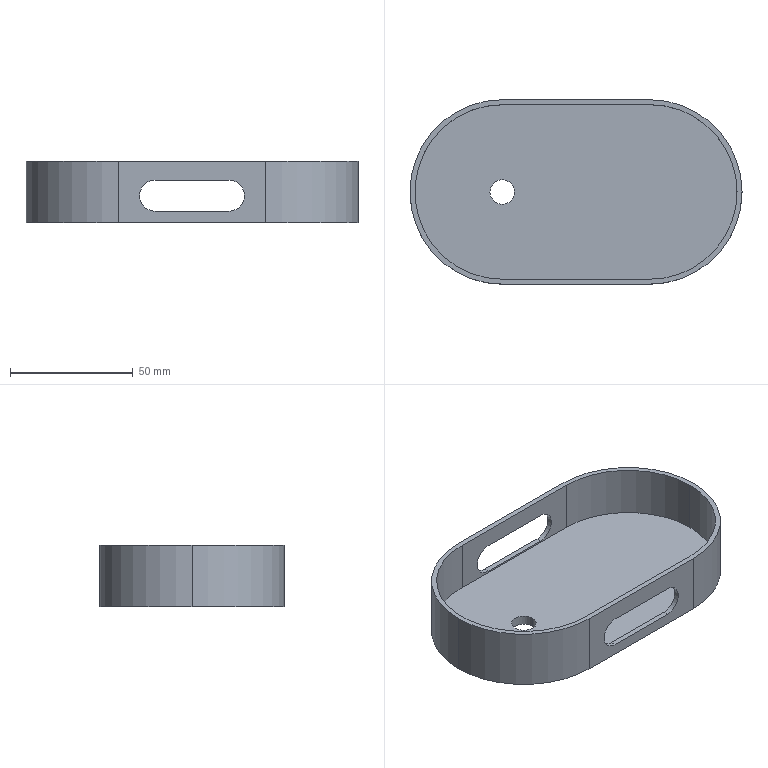Part | SolidWorks | features ICE 2, Extrusion 1, MirrorPattern 1 | 1 solid | 23 faces | box 135 x 75 x 25 mm | volume 48002 mm3 | cylinder 12 | plane 11 | commonest cylinder face diameters 12.684 x4 71 x3 75 x3 10 x2
STEP:
#1=CARTESIAN_POINT('',(95.5,0.,4.));
#2=VERTEX_POINT('',#1);
#3=CARTESIAN_POINT('',(60.,35.5,4.));
#4=VERTEX_POINT('',#3);
#5=CARTESIAN_POINT('',(60.,0.,4.));
#6=DIRECTION('',(0.,0.,1.));
#7=DIRECTION('',(1.,0.,0.));
#8=AXIS2_PLACEMENT_3D('',#5,#6,#7);
#9=CIRCLE('',#8,35.5);
#10=EDGE_CURVE('',#2,#4,#9,.T.);
#11=ORIENTED_EDGE('',*,*,#10,.F.);
#12=CARTESIAN_POINT('',(95.5,0.,25.));
#13=VERTEX_POINT('',#12);
#14=CARTESIAN_POINT('',(95.5,0.,4.));
#15=DIRECTION('',(0.,0.,1.));
#16=VECTOR('',#15,1000.);
#17=LINE('',#14,#16);
#18=EDGE_CURVE('',#2,#13,#17,.T.);
#19=ORIENTED_EDGE('',*,*,#18,.T.);
#20=CARTESIAN_POINT('',(60.,35.5,25.));
#21=VERTEX_POINT('',#20);
#22=CARTESIAN_POINT('',(60.,0.,25.));
#23=DIRECTION('',(0.,0.,1.));
#24=DIRECTION('',(1.,0.,0.));
#25=AXIS2_PLACEMENT_3D('',#22,#23,#24);
#26=CIRCLE('',#25,35.5);
#27=EDGE_CURVE('',#13,#21,#26,.T.);
#28=ORIENTED_EDGE('',*,*,#27,.T.);
#29=CARTESIAN_POINT('',(60.,35.5,4.));
#30=DIRECTION('',(0.,0.,1.));
#31=VECTOR('',#30,1000.);
#32=LINE('',#29,#31);
#33=EDGE_CURVE('',#4,#21,#32,.T.);
#34=ORIENTED_EDGE('',*,*,#33,.F.);
#35=EDGE_LOOP('',(#11,#19,#28,#34));
#36=FACE_OUTER_BOUND('',#35,.T.);
#37=CARTESIAN_POINT('',(60.,0.,4.));
#38=DIRECTION('',(0.,0.,1.));
#39=DIRECTION('',(1.,0.,0.));
#40=AXIS2_PLACEMENT_3D('',#37,#38,#39);
#41=CYLINDRICAL_SURFACE('',#40,35.5);
#42=ADVANCED_FACE('',(#36),#41,.F.);
#43=CARTESIAN_POINT('',(-37.5,0.,25.));
#44=VERTEX_POINT('',#43);
#45=CARTESIAN_POINT('',(0.,-37.5,25.));
#46=VERTEX_POINT('',#45);
#47=CARTESIAN_POINT('',(0.,0.,25.));
#48=DIRECTION('',(0.,0.,1.));
#49=DIRECTION('',(1.,0.,0.));
#50=AXIS2_PLACEMENT_3D('',#47,#48,#49);
#51=CIRCLE('',#50,37.5);
#52=EDGE_CURVE('',#44,#46,#51,.T.);
#53=ORIENTED_EDGE('',*,*,#52,.F.);
#54=CARTESIAN_POINT('',(-37.5,0.,0.));
#55=VERTEX_POINT('',#54);
#56=CARTESIAN_POINT('',(-37.5,0.,25.));
#57=DIRECTION('',(0.,0.,-1.));
#58=VECTOR('',#57,1000.);
#59=LINE('',#56,#58);
#60=EDGE_CURVE('',#44,#55,#59,.T.);
#61=ORIENTED_EDGE('',*,*,#60,.T.);
#62=CARTESIAN_POINT('',(0.,-37.5,0.));
#63=VERTEX_POINT('',#62);
#64=CARTESIAN_POINT('',(0.,0.,0.));
#65=DIRECTION('',(0.,0.,1.));
#66=DIRECTION('',(1.,0.,0.));
#67=AXIS2_PLACEMENT_3D('',#64,#65,#66);
#68=CIRCLE('',#67,37.5);
#69=EDGE_CURVE('',#55,#63,#68,.T.);
#70=ORIENTED_EDGE('',*,*,#69,.T.);
#71=CARTESIAN_POINT('',(0.,-37.5,25.));
#72=DIRECTION('',(0.,0.,-1.));
#73=VECTOR('',#72,1000.);
#74=LINE('',#71,#73);
#75=EDGE_CURVE('',#46,#63,#74,.T.);
#76=ORIENTED_EDGE('',*,*,#75,.F.);
#77=EDGE_LOOP('',(#53,#61,#70,#76));
#78=FACE_OUTER_BOUND('',#77,.T.);
#79=CARTESIAN_POINT('',(0.,0.,25.));
#80=DIRECTION('',(0.,0.,-1.));
#81=DIRECTION('',(-1.,0.,0.));
#82=AXIS2_PLACEMENT_3D('',#79,#80,#81);
#83=CYLINDRICAL_SURFACE('',#82,37.5);
#84=ADVANCED_FACE('',(#78),#83,.T.);
#85=CARTESIAN_POINT('',(-5.,0.,4.));
#86=VERTEX_POINT('',#85);
#87=CARTESIAN_POINT('',(5.,0.,4.));
#88=VERTEX_POINT('',#87);
#89=CARTESIAN_POINT('',(0.,0.,4.));
#90=DIRECTION('',(0.,0.,1.));
#91=DIRECTION('',(1.,0.,0.));
#92=AXIS2_PLACEMENT_3D('',#89,#90,#91);
#93=CIRCLE('',#92,5.);
#94=EDGE_CURVE('',#86,#88,#93,.T.);
#95=ORIENTED_EDGE('',*,*,#94,.T.);
#96=CARTESIAN_POINT('',(5.,0.,0.));
#97=VERTEX_POINT('',#96);
#98=CARTESIAN_POINT('',(5.,0.,25.));
#99=DIRECTION('',(0.,0.,-1.));
#100=VECTOR('',#99,1000.);
#101=LINE('',#98,#100);
#102=EDGE_CURVE('',#88,#97,#101,.T.);
#103=ORIENTED_EDGE('',*,*,#102,.T.);
#104=CARTESIAN_POINT('',(-5.,0.,0.));
#105=VERTEX_POINT('',#104);
#106=CARTESIAN_POINT('',(0.,0.,0.));
#107=DIRECTION('',(0.,0.,1.));
#108=DIRECTION('',(1.,0.,0.));
#109=AXIS2_PLACEMENT_3D('',#106,#107,#108);
#110=CIRCLE('',#109,5.);
#111=EDGE_CURVE('',#105,#97,#110,.T.);
#112=ORIENTED_EDGE('',*,*,#111,.F.);
#113=CARTESIAN_POINT('',(-5.,0.,25.));
#114=DIRECTION('',(0.,0.,-1.));
#115=VECTOR('',#114,1000.);
#116=LINE('',#113,#115);
#117=EDGE_CURVE('',#86,#105,#116,.T.);
#118=ORIENTED_EDGE('',*,*,#117,.F.);
#119=EDGE_LOOP('',(#95,#103,#112,#118));
#120=FACE_OUTER_BOUND('',#119,.T.);
#121=CARTESIAN_POINT('',(0.,0.,25.));
#122=DIRECTION('',(0.,0.,-1.));
#123=DIRECTION('',(-1.,0.,0.));
#124=AXIS2_PLACEMENT_3D('',#121,#122,#123);
#125=CYLINDRICAL_SURFACE('',#124,5.);
#126=ADVANCED_FACE('',(#120),#125,.F.);
#127=CARTESIAN_POINT('',(60.,37.5,0.));
#128=VERTEX_POINT('',#127);
#129=CARTESIAN_POINT('',(0.,37.5,0.));
#130=VERTEX_POINT('',#129);
#131=CARTESIAN_POINT('',(0.,37.5,0.));
#132=DIRECTION('',(-1.,0.,0.));
#133=VECTOR('',#132,1000.);
#134=LINE('',#131,#133);
#135=EDGE_CURVE('',#128,#130,#134,.T.);
#136=ORIENTED_EDGE('',*,*,#135,.T.);
#137=CARTESIAN_POINT('',(0.,37.5,25.));
#138=VERTEX_POINT('',#137);
#139=CARTESIAN_POINT('',(0.,37.5,25.));
#140=DIRECTION('',(0.,0.,-1.));
#141=VECTOR('',#140,1000.);
#142=LINE('',#139,#141);
#143=EDGE_CURVE('',#138,#130,#142,.T.);
#144=ORIENTED_EDGE('',*,*,#143,.F.);
#145=CARTESIAN_POINT('',(60.,37.5,25.));
#146=VERTEX_POINT('',#145);
#147=CARTESIAN_POINT('',(0.,37.5,25.));
#148=DIRECTION('',(-1.,0.,0.));
#149=VECTOR('',#148,1000.);
#150=LINE('',#147,#149);
#151=EDGE_CURVE('',#146,#138,#150,.T.);
#152=ORIENTED_EDGE('',*,*,#151,.F.);
#153=CARTESIAN_POINT('',(60.,37.5,25.));
#154=DIRECTION('',(0.,0.,-1.));
#155=VECTOR('',#154,1000.);
#156=LINE('',#153,#155);
#157=EDGE_CURVE('',#146,#128,#156,.T.);
#158=ORIENTED_EDGE('',*,*,#157,.T.);
#159=EDGE_LOOP('',(#136,#144,#152,#158));
#160=FACE_OUTER_BOUND('',#159,.T.);
#161=CARTESIAN_POINT('',(15.,37.5,17.342));
#162=VERTEX_POINT('',#161);
#163=CARTESIAN_POINT('',(15.,37.5,4.658));
#164=VERTEX_POINT('',#163);
#165=CARTESIAN_POINT('',(15.,37.5,11.));
#166=DIRECTION('',(0.,-1.,0.));
#167=DIRECTION('',(0.,0.,-1.));
#168=AXIS2_PLACEMENT_3D('',#165,#166,#167);
#169=CIRCLE('',#168,6.342);
#170=EDGE_CURVE('',#162,#164,#169,.T.);
#171=ORIENTED_EDGE('',*,*,#170,.T.);
#172=CARTESIAN_POINT('',(45.,37.5,4.658));
#173=VERTEX_POINT('',#172);
#174=CARTESIAN_POINT('',(15.,37.5,4.658));
#175=DIRECTION('',(1.,0.,0.));
#176=VECTOR('',#175,1000.);
#177=LINE('',#174,#176);
#178=EDGE_CURVE('',#164,#173,#177,.T.);
#179=ORIENTED_EDGE('',*,*,#178,.T.);
#180=CARTESIAN_POINT('',(45.,37.5,17.342));
#181=VERTEX_POINT('',#180);
#182=CARTESIAN_POINT('',(45.,37.5,11.));
#183=DIRECTION('',(0.,-1.,0.));
#184=DIRECTION('',(0.,0.,-1.));
#185=AXIS2_PLACEMENT_3D('',#182,#183,#184);
#186=CIRCLE('',#185,6.342);
#187=EDGE_CURVE('',#173,#181,#186,.T.);
#188=ORIENTED_EDGE('',*,*,#187,.T.);
#189=CARTESIAN_POINT('',(15.,37.5,17.342));
#190=DIRECTION('',(-1.,0.,0.));
#191=VECTOR('',#190,1000.);
#192=LINE('',#189,#191);
#193=EDGE_CURVE('',#181,#162,#192,.T.);
#194=ORIENTED_EDGE('',*,*,#193,.T.);
#195=EDGE_LOOP('',(#171,#179,#188,#194));
#196=FACE_BOUND('',#195,.T.);
#197=CARTESIAN_POINT('',(0.,37.5,25.));
#198=DIRECTION('',(0.,-1.,0.));
#199=DIRECTION('',(0.,0.,-1.));
#200=AXIS2_PLACEMENT_3D('',#197,#198,#199);
#201=PLANE('',#200);
#202=ADVANCED_FACE('',(#160,#196),#201,.F.);
#203=CARTESIAN_POINT('',(0.,35.5,25.));
#204=VERTEX_POINT('',#203);
#205=CARTESIAN_POINT('',(60.,35.5,25.));
#206=DIRECTION('',(-1.,0.,0.));
#207=VECTOR('',#206,1000.);
#208=LINE('',#205,#207);
#209=EDGE_CURVE('',#21,#204,#208,.T.);
#210=ORIENTED_EDGE('',*,*,#209,.T.);
#211=CARTESIAN_POINT('',(0.,35.5,4.));
#212=VERTEX_POINT('',#211);
#213=CARTESIAN_POINT('',(0.,35.5,4.));
#214=DIRECTION('',(0.,0.,1.));
#215=VECTOR('',#214,1000.);
#216=LINE('',#213,#215);
#217=EDGE_CURVE('',#212,#204,#216,.T.);
#218=ORIENTED_EDGE('',*,*,#217,.F.);
#219=CARTESIAN_POINT('',(60.,35.5,4.));
#220=DIRECTION('',(-1.,0.,0.));
#221=VECTOR('',#220,1000.);
#222=LINE('',#219,#221);
#223=EDGE_CURVE('',#4,#212,#222,.T.);
#224=ORIENTED_EDGE('',*,*,#223,.F.);
#225=ORIENTED_EDGE('',*,*,#33,.T.);
#226=EDGE_LOOP('',(#210,#218,#224,#225));
#227=FACE_OUTER_BOUND('',#226,.T.);
#228=CARTESIAN_POINT('',(15.,35.5,17.342));
#229=VERTEX_POINT('',#228);
#230=CARTESIAN_POINT('',(15.,35.5,4.658));
#231=VERTEX_POINT('',#230);
#232=CARTESIAN_POINT('',(15.,35.5,11.));
#233=DIRECTION('',(0.,-1.,0.));
#234=DIRECTION('',(0.,0.,1.));
#235=AXIS2_PLACEMENT_3D('',#232,#233,#234);
#236=CIRCLE('',#235,6.342);
#237=EDGE_CURVE('',#229,#231,#236,.T.);
#238=ORIENTED_EDGE('',*,*,#237,.F.);
#239=CARTESIAN_POINT('',(45.,35.5,17.342));
#240=VERTEX_POINT('',#239);
#241=CARTESIAN_POINT('',(60.,35.5,17.342));
#242=DIRECTION('',(-1.,0.,0.));
#243=VECTOR('',#242,1000.);
#244=LINE('',#241,#243);
#245=EDGE_CURVE('',#240,#229,#244,.T.);
#246=ORIENTED_EDGE('',*,*,#245,.F.);
#247=CARTESIAN_POINT('',(45.,35.5,4.658));
#248=VERTEX_POINT('',#247);
#249=CARTESIAN_POINT('',(45.,35.5,11.));
#250=DIRECTION('',(0.,-1.,0.));
#251=DIRECTION('',(0.,0.,1.));
#252=AXIS2_PLACEMENT_3D('',#249,#250,#251);
#253=CIRCLE('',#252,6.342);
#254=EDGE_CURVE('',#248,#240,#253,.T.);
#255=ORIENTED_EDGE('',*,*,#254,.F.);
#256=CARTESIAN_POINT('',(60.,35.5,4.658));
#257=DIRECTION('',(1.,0.,0.));
#258=VECTOR('',#257,1000.);
#259=LINE('',#256,#258);
#260=EDGE_CURVE('',#231,#248,#259,.T.);
#261=ORIENTED_EDGE('',*,*,#260,.F.);
#262=EDGE_LOOP('',(#238,#246,#255,#261));
#263=FACE_BOUND('',#262,.T.);
#264=CARTESIAN_POINT('',(60.,35.5,4.));
#265=DIRECTION('',(0.,1.,0.));
#266=DIRECTION('',(0.,0.,1.));
#267=AXIS2_PLACEMENT_3D('',#264,#265,#266);
#268=PLANE('',#267);
#269=ADVANCED_FACE('',(#227,#263),#268,.F.);
#270=ORIENTED_EDGE('',*,*,#102,.F.);
#271=CARTESIAN_POINT('',(0.,0.,4.));
#272=DIRECTION('',(0.,0.,1.));
#273=DIRECTION('',(1.,0.,0.));
#274=AXIS2_PLACEMENT_3D('',#271,#272,#273);
#275=CIRCLE('',#274,5.);
#276=EDGE_CURVE('',#88,#86,#275,.T.);
#277=ORIENTED_EDGE('',*,*,#276,.T.);
#278=ORIENTED_EDGE('',*,*,#117,.T.);
#279=CARTESIAN_POINT('',(0.,0.,0.));
#280=DIRECTION('',(0.,0.,1.));
#281=DIRECTION('',(1.,0.,0.));
#282=AXIS2_PLACEMENT_3D('',#279,#280,#281);
#283=CIRCLE('',#282,5.);
#284=EDGE_CURVE('',#97,#105,#283,.T.);
#285=ORIENTED_EDGE('',*,*,#284,.F.);
#286=EDGE_LOOP('',(#270,#277,#278,#285));
#287=FACE_OUTER_BOUND('',#286,.T.);
#288=CARTESIAN_POINT('',(0.,0.,25.));
#289=DIRECTION('',(0.,0.,-1.));
#290=DIRECTION('',(-1.,0.,0.));
#291=AXIS2_PLACEMENT_3D('',#288,#289,#290);
#292=CYLINDRICAL_SURFACE('',#291,5.);
#293=ADVANCED_FACE('',(#287),#292,.F.);
#294=CARTESIAN_POINT('',(60.,-35.5,25.));
#295=VERTEX_POINT('',#294);
#296=CARTESIAN_POINT('',(60.,0.,25.));
#297=DIRECTION('',(0.,0.,1.));
#298=DIRECTION('',(1.,0.,0.));
#299=AXIS2_PLACEMENT_3D('',#296,#297,#298);
#300=CIRCLE('',#299,35.5);
#301=EDGE_CURVE('',#295,#13,#300,.T.);
#302=ORIENTED_EDGE('',*,*,#301,.F.);
#303=CARTESIAN_POINT('',(0.,-35.5,25.));
#304=VERTEX_POINT('',#303);
#305=CARTESIAN_POINT('',(0.,-35.5,25.));
#306=DIRECTION('',(1.,0.,0.));
#307=VECTOR('',#306,1000.);
#308=LINE('',#305,#307);
#309=EDGE_CURVE('',#304,#295,#308,.T.);
#310=ORIENTED_EDGE('',*,*,#309,.F.);
#311=CARTESIAN_POINT('',(0.,0.,25.));
#312=DIRECTION('',(0.,0.,1.));
#313=DIRECTION('',(1.,0.,0.));
#314=AXIS2_PLACEMENT_3D('',#311,#312,#313);
#315=CIRCLE('',#314,35.5);
#316=EDGE_CURVE('',#204,#304,#315,.T.);
#317=ORIENTED_EDGE('',*,*,#316,.F.);
#318=ORIENTED_EDGE('',*,*,#209,.F.);
#319=ORIENTED_EDGE('',*,*,#27,.F.);
#320=EDGE_LOOP('',(#302,#310,#317,#318,#319));
#321=FACE_BOUND('',#320,.T.);
#322=CARTESIAN_POINT('',(60.,-37.5,25.));
#323=VERTEX_POINT('',#322);
#324=CARTESIAN_POINT('',(60.,0.,25.));
#325=DIRECTION('',(0.,0.,1.));
#326=DIRECTION('',(1.,0.,0.));
#327=AXIS2_PLACEMENT_3D('',#324,#325,#326);
#328=CIRCLE('',#327,37.5);
#329=EDGE_CURVE('',#323,#146,#328,.T.);
#330=ORIENTED_EDGE('',*,*,#329,.T.);
#331=ORIENTED_EDGE('',*,*,#151,.T.);
#332=CARTESIAN_POINT('',(0.,0.,25.));
#333=DIRECTION('',(0.,0.,1.));
#334=DIRECTION('',(1.,0.,0.));
#335=AXIS2_PLACEMENT_3D('',#332,#333,#334);
#336=CIRCLE('',#335,37.5);
#337=EDGE_CURVE('',#138,#44,#336,.T.);
#338=ORIENTED_EDGE('',*,*,#337,.T.);
#339=ORIENTED_EDGE('',*,*,#52,.T.);
#340=CARTESIAN_POINT('',(0.,-37.5,25.));
#341=DIRECTION('',(1.,0.,0.));
#342=VECTOR('',#341,1000.);
#343=LINE('',#340,#342);
#344=EDGE_CURVE('',#46,#323,#343,.T.);
#345=ORIENTED_EDGE('',*,*,#344,.T.);
#346=EDGE_LOOP('',(#330,#331,#338,#339,#345));
#347=FACE_OUTER_BOUND('',#346,.T.);
#348=CARTESIAN_POINT('',(60.,0.,25.));
#349=DIRECTION('',(0.,0.,1.));
#350=DIRECTION('',(1.,0.,0.));
#351=AXIS2_PLACEMENT_3D('',#348,#349,#350);
#352=PLANE('',#351);
#353=ADVANCED_FACE('',(#321,#347),#352,.T.);
#354=CARTESIAN_POINT('',(60.,-37.5,0.));
#355=VERTEX_POINT('',#354);
#356=CARTESIAN_POINT('',(60.,0.,0.));
#357=DIRECTION('',(0.,0.,1.));
#358=DIRECTION('',(1.,0.,0.));
#359=AXIS2_PLACEMENT_3D('',#356,#357,#358);
#360=CIRCLE('',#359,37.5);
#361=EDGE_CURVE('',#355,#128,#360,.T.);
#362=ORIENTED_EDGE('',*,*,#361,.F.);
#363=CARTESIAN_POINT('',(0.,-37.5,0.));
#364=DIRECTION('',(1.,0.,0.));
#365=VECTOR('',#364,1000.);
#366=LINE('',#363,#365);
#367=EDGE_CURVE('',#63,#355,#366,.T.);
#368=ORIENTED_EDGE('',*,*,#367,.F.);
#369=ORIENTED_EDGE('',*,*,#69,.F.);
#370=CARTESIAN_POINT('',(0.,0.,0.));
#371=DIRECTION('',(0.,0.,1.));
#372=DIRECTION('',(1.,0.,0.));
#373=AXIS2_PLACEMENT_3D('',#370,#371,#372);
#374=CIRCLE('',#373,37.5);
#375=EDGE_CURVE('',#130,#55,#374,.T.);
#376=ORIENTED_EDGE('',*,*,#375,.F.);
#377=ORIENTED_EDGE('',*,*,#135,.F.);
#378=EDGE_LOOP('',(#362,#368,#369,#376,#377));
#379=FACE_OUTER_BOUND('',#378,.T.);
#380=ORIENTED_EDGE('',*,*,#111,.T.);
#381=ORIENTED_EDGE('',*,*,#284,.T.);
#382=EDGE_LOOP('',(#380,#381));
#383=FACE_BOUND('',#382,.T.);
#384=CARTESIAN_POINT('',(60.,0.,0.));
#385=DIRECTION('',(0.,0.,1.));
#386=DIRECTION('',(1.,0.,0.));
#387=AXIS2_PLACEMENT_3D('',#384,#385,#386);
#388=PLANE('',#387);
#389=ADVANCED_FACE('',(#379,#383),#388,.F.);
#390=ORIENTED_EDGE('',*,*,#361,.T.);
#391=ORIENTED_EDGE('',*,*,#157,.F.);
#392=ORIENTED_EDGE('',*,*,#329,.F.);
#393=CARTESIAN_POINT('',(60.,-37.5,25.));
#394=DIRECTION('',(0.,0.,-1.));
#395=VECTOR('',#394,1000.);
#396=LINE('',#393,#395);
#397=EDGE_CURVE('',#323,#355,#396,.T.);
#398=ORIENTED_EDGE('',*,*,#397,.T.);
#399=EDGE_LOOP('',(#390,#391,#392,#398));
#400=FACE_OUTER_BOUND('',#399,.T.);
#401=CARTESIAN_POINT('',(60.,0.,25.));
#402=DIRECTION('',(0.,0.,-1.));
#403=DIRECTION('',(-1.,0.,0.));
#404=AXIS2_PLACEMENT_3D('',#401,#402,#403);
#405=CYLINDRICAL_SURFACE('',#404,37.5);
#406=ADVANCED_FACE('',(#400),#405,.T.);
#407=ORIENTED_EDGE('',*,*,#60,.F.);
#408=ORIENTED_EDGE('',*,*,#337,.F.);
#409=ORIENTED_EDGE('',*,*,#143,.T.);
#410=ORIENTED_EDGE('',*,*,#375,.T.);
#411=EDGE_LOOP('',(#407,#408,#409,#410));
#412=FACE_OUTER_BOUND('',#411,.T.);
#413=CARTESIAN_POINT('',(0.,0.,25.));
#414=DIRECTION('',(0.,0.,-1.));
#415=DIRECTION('',(-1.,0.,0.));
#416=AXIS2_PLACEMENT_3D('',#413,#414,#415);
#417=CYLINDRICAL_SURFACE('',#416,37.5);
#418=ADVANCED_FACE('',(#412),#417,.T.);
#419=CARTESIAN_POINT('',(15.,-37.5,4.658));
#420=VERTEX_POINT('',#419);
#421=CARTESIAN_POINT('',(45.,-37.5,4.658));
#422=VERTEX_POINT('',#421);
#423=CARTESIAN_POINT('',(15.,-37.5,4.658));
#424=DIRECTION('',(1.,0.,0.));
#425=VECTOR('',#424,1000.);
#426=LINE('',#423,#425);
#427=EDGE_CURVE('',#420,#422,#426,.T.);
#428=ORIENTED_EDGE('',*,*,#427,.F.);
#429=CARTESIAN_POINT('',(15.,-37.5,17.342));
#430=VERTEX_POINT('',#429);
#431=CARTESIAN_POINT('',(15.,-37.5,11.));
#432=DIRECTION('',(0.,-1.,0.));
#433=DIRECTION('',(0.,0.,-1.));
#434=AXIS2_PLACEMENT_3D('',#431,#432,#433);
#435=CIRCLE('',#434,6.342);
#436=EDGE_CURVE('',#430,#420,#435,.T.);
#437=ORIENTED_EDGE('',*,*,#436,.F.);
#438=CARTESIAN_POINT('',(45.,-37.5,17.342));
#439=VERTEX_POINT('',#438);
#440=CARTESIAN_POINT('',(15.,-37.5,17.342));
#441=DIRECTION('',(-1.,0.,0.));
#442=VECTOR('',#441,1000.);
#443=LINE('',#440,#442);
#444=EDGE_CURVE('',#439,#430,#443,.T.);
#445=ORIENTED_EDGE('',*,*,#444,.F.);
#446=CARTESIAN_POINT('',(45.,-37.5,11.));
#447=DIRECTION('',(0.,-1.,0.));
#448=DIRECTION('',(0.,0.,-1.));
#449=AXIS2_PLACEMENT_3D('',#446,#447,#448);
#450=CIRCLE('',#449,6.342);
#451=EDGE_CURVE('',#422,#439,#450,.T.);
#452=ORIENTED_EDGE('',*,*,#451,.F.);
#453=EDGE_LOOP('',(#428,#437,#445,#452));
#454=FACE_BOUND('',#453,.T.);
#455=ORIENTED_EDGE('',*,*,#367,.T.);
#456=ORIENTED_EDGE('',*,*,#397,.F.);
#457=ORIENTED_EDGE('',*,*,#344,.F.);
#458=ORIENTED_EDGE('',*,*,#75,.T.);
#459=EDGE_LOOP('',(#455,#456,#457,#458));
#460=FACE_OUTER_BOUND('',#459,.T.);
#461=CARTESIAN_POINT('',(0.,-37.5,25.));
#462=DIRECTION('',(0.,1.,0.));
#463=DIRECTION('',(0.,0.,1.));
#464=AXIS2_PLACEMENT_3D('',#461,#462,#463);
#465=PLANE('',#464);
#466=ADVANCED_FACE('',(#454,#460),#465,.F.);
#467=ORIENTED_EDGE('',*,*,#18,.F.);
#468=CARTESIAN_POINT('',(60.,-35.5,4.));
#469=VERTEX_POINT('',#468);
#470=CARTESIAN_POINT('',(60.,0.,4.));
#471=DIRECTION('',(0.,0.,1.));
#472=DIRECTION('',(1.,0.,0.));
#473=AXIS2_PLACEMENT_3D('',#470,#471,#472);
#474=CIRCLE('',#473,35.5);
#475=EDGE_CURVE('',#469,#2,#474,.T.);
#476=ORIENTED_EDGE('',*,*,#475,.F.);
#477=CARTESIAN_POINT('',(60.,-35.5,4.));
#478=DIRECTION('',(0.,0.,1.));
#479=VECTOR('',#478,1000.);
#480=LINE('',#477,#479);
#481=EDGE_CURVE('',#469,#295,#480,.T.);
#482=ORIENTED_EDGE('',*,*,#481,.T.);
#483=ORIENTED_EDGE('',*,*,#301,.T.);
#484=EDGE_LOOP('',(#467,#476,#482,#483));
#485=FACE_OUTER_BOUND('',#484,.T.);
#486=CARTESIAN_POINT('',(60.,0.,4.));
#487=DIRECTION('',(0.,0.,1.));
#488=DIRECTION('',(1.,0.,0.));
#489=AXIS2_PLACEMENT_3D('',#486,#487,#488);
#490=CYLINDRICAL_SURFACE('',#489,35.5);
#491=ADVANCED_FACE('',(#485),#490,.F.);
#492=CARTESIAN_POINT('',(45.,-35.5,17.342));
#493=VERTEX_POINT('',#492);
#494=CARTESIAN_POINT('',(15.,-35.5,17.342));
#495=VERTEX_POINT('',#494);
#496=CARTESIAN_POINT('',(0.,-35.5,17.342));
#497=DIRECTION('',(-1.,0.,0.));
#498=VECTOR('',#497,1000.);
#499=LINE('',#496,#498);
#500=EDGE_CURVE('',#493,#495,#499,.T.);
#501=ORIENTED_EDGE('',*,*,#500,.T.);
#502=CARTESIAN_POINT('',(15.,-35.5,4.658));
#503=VERTEX_POINT('',#502);
#504=CARTESIAN_POINT('',(15.,-35.5,11.));
#505=DIRECTION('',(0.,-1.,0.));
#506=DIRECTION('',(0.,0.,-1.));
#507=AXIS2_PLACEMENT_3D('',#504,#505,#506);
#508=CIRCLE('',#507,6.342);
#509=EDGE_CURVE('',#495,#503,#508,.T.);
#510=ORIENTED_EDGE('',*,*,#509,.T.);
#511=CARTESIAN_POINT('',(45.,-35.5,4.658));
#512=VERTEX_POINT('',#511);
#513=CARTESIAN_POINT('',(0.,-35.5,4.658));
#514=DIRECTION('',(1.,0.,0.));
#515=VECTOR('',#514,1000.);
#516=LINE('',#513,#515);
#517=EDGE_CURVE('',#503,#512,#516,.T.);
#518=ORIENTED_EDGE('',*,*,#517,.T.);
#519=CARTESIAN_POINT('',(45.,-35.5,11.));
#520=DIRECTION('',(0.,-1.,0.));
#521=DIRECTION('',(0.,0.,-1.));
#522=AXIS2_PLACEMENT_3D('',#519,#520,#521);
#523=CIRCLE('',#522,6.342);
#524=EDGE_CURVE('',#512,#493,#523,.T.);
#525=ORIENTED_EDGE('',*,*,#524,.T.);
#526=EDGE_LOOP('',(#501,#510,#518,#525));
#527=FACE_BOUND('',#526,.T.);
#528=ORIENTED_EDGE('',*,*,#309,.T.);
#529=ORIENTED_EDGE('',*,*,#481,.F.);
#530=CARTESIAN_POINT('',(0.,-35.5,4.));
#531=VERTEX_POINT('',#530);
#532=CARTESIAN_POINT('',(0.,-35.5,4.));
#533=DIRECTION('',(1.,0.,0.));
#534=VECTOR('',#533,1000.);
#535=LINE('',#532,#534);
#536=EDGE_CURVE('',#531,#469,#535,.T.);
#537=ORIENTED_EDGE('',*,*,#536,.F.);
#538=CARTESIAN_POINT('',(0.,-35.5,4.));
#539=DIRECTION('',(0.,0.,1.));
#540=VECTOR('',#539,1000.);
#541=LINE('',#538,#540);
#542=EDGE_CURVE('',#531,#304,#541,.T.);
#543=ORIENTED_EDGE('',*,*,#542,.T.);
#544=EDGE_LOOP('',(#528,#529,#537,#543));
#545=FACE_OUTER_BOUND('',#544,.T.);
#546=CARTESIAN_POINT('',(0.,-35.5,4.));
#547=DIRECTION('',(0.,-1.,0.));
#548=DIRECTION('',(0.,0.,-1.));
#549=AXIS2_PLACEMENT_3D('',#546,#547,#548);
#550=PLANE('',#549);
#551=ADVANCED_FACE('',(#527,#545),#550,.F.);
#552=ORIENTED_EDGE('',*,*,#316,.T.);
#553=ORIENTED_EDGE('',*,*,#542,.F.);
#554=CARTESIAN_POINT('',(0.,0.,4.));
#555=DIRECTION('',(0.,0.,1.));
#556=DIRECTION('',(1.,0.,0.));
#557=AXIS2_PLACEMENT_3D('',#554,#555,#556);
#558=CIRCLE('',#557,35.5);
#559=EDGE_CURVE('',#212,#531,#558,.T.);
#560=ORIENTED_EDGE('',*,*,#559,.F.);
#561=ORIENTED_EDGE('',*,*,#217,.T.);
#562=EDGE_LOOP('',(#552,#553,#560,#561));
#563=FACE_OUTER_BOUND('',#562,.T.);
#564=CARTESIAN_POINT('',(0.,0.,4.));
#565=DIRECTION('',(0.,0.,1.));
#566=DIRECTION('',(1.,0.,0.));
#567=AXIS2_PLACEMENT_3D('',#564,#565,#566);
#568=CYLINDRICAL_SURFACE('',#567,35.5);
#569=ADVANCED_FACE('',(#563),#568,.F.);
#570=ORIENTED_EDGE('',*,*,#94,.F.);
#571=ORIENTED_EDGE('',*,*,#276,.F.);
#572=EDGE_LOOP('',(#570,#571));
#573=FACE_BOUND('',#572,.T.);
#574=ORIENTED_EDGE('',*,*,#475,.T.);
#575=ORIENTED_EDGE('',*,*,#10,.T.);
#576=ORIENTED_EDGE('',*,*,#223,.T.);
#577=ORIENTED_EDGE('',*,*,#559,.T.);
#578=ORIENTED_EDGE('',*,*,#536,.T.);
#579=EDGE_LOOP('',(#574,#575,#576,#577,#578));
#580=FACE_OUTER_BOUND('',#579,.T.);
#581=CARTESIAN_POINT('',(60.,0.,4.));
#582=DIRECTION('',(0.,0.,1.));
#583=DIRECTION('',(1.,0.,0.));
#584=AXIS2_PLACEMENT_3D('',#581,#582,#583);
#585=PLANE('',#584);
#586=ADVANCED_FACE('',(#573,#580),#585,.T.);
#587=CARTESIAN_POINT('',(15.,-16.5,17.342));
#588=DIRECTION('',(0.,-1.,0.));
#589=VECTOR('',#588,1000.);
#590=LINE('',#587,#589);
#591=EDGE_CURVE('',#495,#430,#590,.T.);
#592=ORIENTED_EDGE('',*,*,#591,.T.);
#593=ORIENTED_EDGE('',*,*,#436,.T.);
#594=CARTESIAN_POINT('',(15.,-16.5,4.658));
#595=DIRECTION('',(0.,-1.,0.));
#596=VECTOR('',#595,1000.);
#597=LINE('',#594,#596);
#598=EDGE_CURVE('',#503,#420,#597,.T.);
#599=ORIENTED_EDGE('',*,*,#598,.F.);
#600=ORIENTED_EDGE('',*,*,#509,.F.);
#601=EDGE_LOOP('',(#592,#593,#599,#600));
#602=FACE_OUTER_BOUND('',#601,.T.);
#603=CARTESIAN_POINT('',(15.,-16.5,11.));
#604=DIRECTION('',(0.,-1.,0.));
#605=DIRECTION('',(0.,0.,-1.));
#606=AXIS2_PLACEMENT_3D('',#603,#604,#605);
#607=CYLINDRICAL_SURFACE('',#606,6.342);
#608=ADVANCED_FACE('',(#602),#607,.F.);
#609=CARTESIAN_POINT('',(45.,-16.5,17.342));
#610=DIRECTION('',(0.,-1.,0.));
#611=VECTOR('',#610,1000.);
#612=LINE('',#609,#611);
#613=EDGE_CURVE('',#493,#439,#612,.T.);
#614=ORIENTED_EDGE('',*,*,#613,.T.);
#615=ORIENTED_EDGE('',*,*,#444,.T.);
#616=ORIENTED_EDGE('',*,*,#591,.F.);
#617=ORIENTED_EDGE('',*,*,#500,.F.);
#618=EDGE_LOOP('',(#614,#615,#616,#617));
#619=FACE_OUTER_BOUND('',#618,.T.);
#620=CARTESIAN_POINT('',(15.,-16.5,17.342));
#621=DIRECTION('',(0.,0.,1.));
#622=DIRECTION('',(1.,0.,0.));
#623=AXIS2_PLACEMENT_3D('',#620,#621,#622);
#624=PLANE('',#623);
#625=ADVANCED_FACE('',(#619),#624,.F.);
#626=CARTESIAN_POINT('',(45.,-16.5,4.658));
#627=DIRECTION('',(0.,-1.,0.));
#628=VECTOR('',#627,1000.);
#629=LINE('',#626,#628);
#630=EDGE_CURVE('',#512,#422,#629,.T.);
#631=ORIENTED_EDGE('',*,*,#630,.T.);
#632=ORIENTED_EDGE('',*,*,#451,.T.);
#633=ORIENTED_EDGE('',*,*,#613,.F.);
#634=ORIENTED_EDGE('',*,*,#524,.F.);
#635=EDGE_LOOP('',(#631,#632,#633,#634));
#636=FACE_OUTER_BOUND('',#635,.T.);
#637=CARTESIAN_POINT('',(45.,-16.5,11.));
#638=DIRECTION('',(0.,-1.,0.));
#639=DIRECTION('',(0.,0.,-1.));
#640=AXIS2_PLACEMENT_3D('',#637,#638,#639);
#641=CYLINDRICAL_SURFACE('',#640,6.342);
#642=ADVANCED_FACE('',(#636),#641,.F.);
#643=ORIENTED_EDGE('',*,*,#598,.T.);
#644=ORIENTED_EDGE('',*,*,#427,.T.);
#645=ORIENTED_EDGE('',*,*,#630,.F.);
#646=ORIENTED_EDGE('',*,*,#517,.F.);
#647=EDGE_LOOP('',(#643,#644,#645,#646));
#648=FACE_OUTER_BOUND('',#647,.T.);
#649=CARTESIAN_POINT('',(15.,-16.5,4.658));
#650=DIRECTION('',(0.,0.,-1.));
#651=DIRECTION('',(-1.,0.,0.));
#652=AXIS2_PLACEMENT_3D('',#649,#650,#651);
#653=PLANE('',#652);
#654=ADVANCED_FACE('',(#648),#653,.F.);
#655=ORIENTED_EDGE('',*,*,#237,.T.);
#656=CARTESIAN_POINT('',(15.,16.5,4.658));
#657=DIRECTION('',(0.,1.,0.));
#658=VECTOR('',#657,1000.);
#659=LINE('',#656,#658);
#660=EDGE_CURVE('',#231,#164,#659,.T.);
#661=ORIENTED_EDGE('',*,*,#660,.T.);
#662=ORIENTED_EDGE('',*,*,#170,.F.);
#663=CARTESIAN_POINT('',(15.,16.5,17.342));
#664=DIRECTION('',(0.,1.,0.));
#665=VECTOR('',#664,1000.);
#666=LINE('',#663,#665);
#667=EDGE_CURVE('',#229,#162,#666,.T.);
#668=ORIENTED_EDGE('',*,*,#667,.F.);
#669=EDGE_LOOP('',(#655,#661,#662,#668));
#670=FACE_OUTER_BOUND('',#669,.T.);
#671=CARTESIAN_POINT('',(15.,16.5,11.));
#672=DIRECTION('',(0.,1.,0.));
#673=DIRECTION('',(0.,0.,1.));
#674=AXIS2_PLACEMENT_3D('',#671,#672,#673);
#675=CYLINDRICAL_SURFACE('',#674,6.342);
#676=ADVANCED_FACE('',(#670),#675,.F.);
#677=ORIENTED_EDGE('',*,*,#260,.T.);
#678=CARTESIAN_POINT('',(45.,16.5,4.658));
#679=DIRECTION('',(0.,1.,0.));
#680=VECTOR('',#679,1000.);
#681=LINE('',#678,#680);
#682=EDGE_CURVE('',#248,#173,#681,.T.);
#683=ORIENTED_EDGE('',*,*,#682,.T.);
#684=ORIENTED_EDGE('',*,*,#178,.F.);
#685=ORIENTED_EDGE('',*,*,#660,.F.);
#686=EDGE_LOOP('',(#677,#683,#684,#685));
#687=FACE_OUTER_BOUND('',#686,.T.);
#688=CARTESIAN_POINT('',(15.,16.5,4.658));
#689=DIRECTION('',(0.,0.,1.));
#690=DIRECTION('',(1.,0.,0.));
#691=AXIS2_PLACEMENT_3D('',#688,#689,#690);
#692=PLANE('',#691);
#693=ADVANCED_FACE('',(#687),#692,.T.);
#694=ORIENTED_EDGE('',*,*,#254,.T.);
#695=CARTESIAN_POINT('',(45.,16.5,17.342));
#696=DIRECTION('',(0.,1.,0.));
#697=VECTOR('',#696,1000.);
#698=LINE('',#695,#697);
#699=EDGE_CURVE('',#240,#181,#698,.T.);
#700=ORIENTED_EDGE('',*,*,#699,.T.);
#701=ORIENTED_EDGE('',*,*,#187,.F.);
#702=ORIENTED_EDGE('',*,*,#682,.F.);
#703=EDGE_LOOP('',(#694,#700,#701,#702));
#704=FACE_OUTER_BOUND('',#703,.T.);
#705=CARTESIAN_POINT('',(45.,16.5,11.));
#706=DIRECTION('',(0.,1.,0.));
#707=DIRECTION('',(0.,0.,1.));
#708=AXIS2_PLACEMENT_3D('',#705,#706,#707);
#709=CYLINDRICAL_SURFACE('',#708,6.342);
#710=ADVANCED_FACE('',(#704),#709,.F.);
#711=ORIENTED_EDGE('',*,*,#245,.T.);
#712=ORIENTED_EDGE('',*,*,#667,.T.);
#713=ORIENTED_EDGE('',*,*,#193,.F.);
#714=ORIENTED_EDGE('',*,*,#699,.F.);
#715=EDGE_LOOP('',(#711,#712,#713,#714));
#716=FACE_OUTER_BOUND('',#715,.T.);
#717=CARTESIAN_POINT('',(15.,16.5,17.342));
#718=DIRECTION('',(0.,0.,-1.));
#719=DIRECTION('',(-1.,0.,0.));
#720=AXIS2_PLACEMENT_3D('',#717,#718,#719);
#721=PLANE('',#720);
#722=ADVANCED_FACE('',(#716),#721,.T.);
#723=CLOSED_SHELL('',(#42,#84,#126,#202,#269,#293,#353,#389,#406,#418,#466,#491,#551,#569,#586,#608,#625,#642,#654,#676,#693,#710,#722));
#724=MANIFOLD_SOLID_BREP('',#723);
#725=CARTESIAN_POINT('',(0.,0.,0.));
#726=DIRECTION('',(0.,0.,1.));
#727=DIRECTION('',(1.,0.,0.));
#728=AXIS2_PLACEMENT_3D('',#725,#726,#727);
#729=(LENGTH_UNIT()NAMED_UNIT(*)SI_UNIT(.MILLI.,.METRE.));
#730=UNCERTAINTY_MEASURE_WITH_UNIT(LENGTH_MEASURE(0.00001),#729,'','');
#731=(NAMED_UNIT(*)PLANE_ANGLE_UNIT()SI_UNIT($,.RADIAN.));
#732=(NAMED_UNIT(*)SI_UNIT($,.STERADIAN.)SOLID_ANGLE_UNIT());
#733=(GEOMETRIC_REPRESENTATION_CONTEXT(3)GLOBAL_UNCERTAINTY_ASSIGNED_CONTEXT((#730))GLOBAL_UNIT_ASSIGNED_CONTEXT((#729,#731,#732))REPRESENTATION_CONTEXT('',''));
#734=ADVANCED_BREP_SHAPE_REPRESENTATION('',(#724,#728),#733);